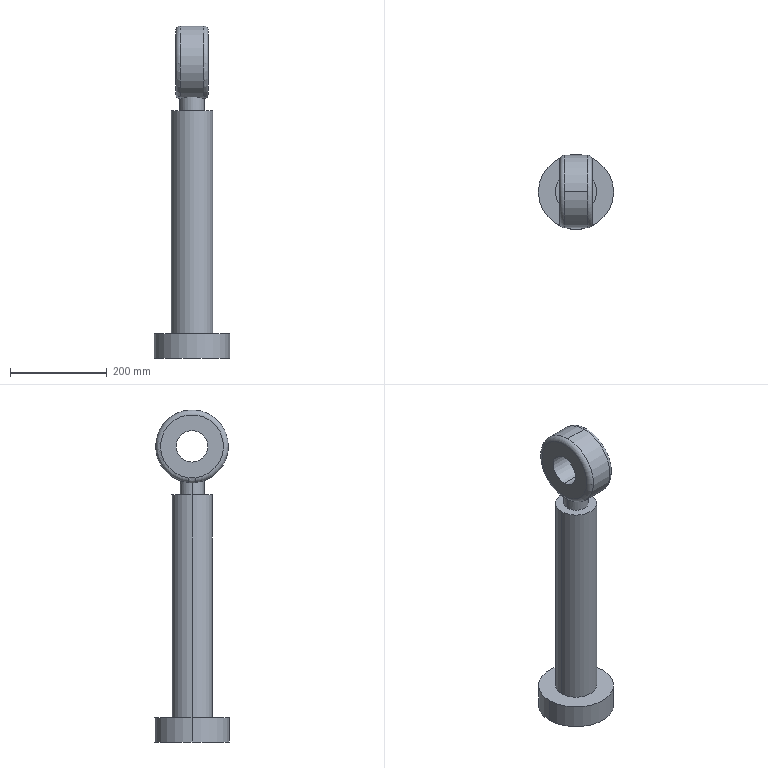Part | SolidWorks | features ICE 3, Extrusion 1, Fillet 1, RevCut 1 | 1 solid | 19 faces | box 155 x 155 x 685 mm | volume 4561292 mm3 | cylinder 10 | plane 5 | torus 2 | spline 2 | commonest cylinder face diameters 50 x2 65 x2 85 x2 150 x2 155 x2
STEP:
#1=CARTESIAN_POINT('',(34.,0.,592.5));
#2=VERTEX_POINT('',#1);
#3=CARTESIAN_POINT('',(34.,0.,527.5));
#4=VERTEX_POINT('',#3);
#5=CARTESIAN_POINT('',(34.,0.,560.));
#6=DIRECTION('',(1.,0.,0.));
#7=DIRECTION('',(0.,0.,-1.));
#8=AXIS2_PLACEMENT_3D('',#5,#6,#7);
#9=CIRCLE('',#8,32.5);
#10=EDGE_CURVE('',#2,#4,#9,.T.);
#11=ORIENTED_EDGE('',*,*,#10,.T.);
#12=CARTESIAN_POINT('',(-34.,0.,527.5));
#13=VERTEX_POINT('',#12);
#14=CARTESIAN_POINT('',(34.,0.,527.5));
#15=DIRECTION('',(-1.,0.,0.));
#16=VECTOR('',#15,1000.);
#17=LINE('',#14,#16);
#18=EDGE_CURVE('',#4,#13,#17,.T.);
#19=ORIENTED_EDGE('',*,*,#18,.T.);
#20=CARTESIAN_POINT('',(-34.,0.,592.5));
#21=VERTEX_POINT('',#20);
#22=CARTESIAN_POINT('',(-34.,0.,560.));
#23=DIRECTION('',(1.,0.,0.));
#24=DIRECTION('',(0.,0.,-1.));
#25=AXIS2_PLACEMENT_3D('',#22,#23,#24);
#26=CIRCLE('',#25,32.5);
#27=EDGE_CURVE('',#21,#13,#26,.T.);
#28=ORIENTED_EDGE('',*,*,#27,.F.);
#29=CARTESIAN_POINT('',(34.,0.,592.5));
#30=DIRECTION('',(-1.,0.,0.));
#31=VECTOR('',#30,1000.);
#32=LINE('',#29,#31);
#33=EDGE_CURVE('',#2,#21,#32,.T.);
#34=ORIENTED_EDGE('',*,*,#33,.F.);
#35=EDGE_LOOP('',(#11,#19,#28,#34));
#36=FACE_OUTER_BOUND('',#35,.T.);
#37=CARTESIAN_POINT('',(34.,0.,560.));
#38=DIRECTION('',(-1.,0.,0.));
#39=DIRECTION('',(0.,0.,1.));
#40=AXIS2_PLACEMENT_3D('',#37,#38,#39);
#41=CYLINDRICAL_SURFACE('',#40,32.5);
#42=ADVANCED_FACE('',(#36),#41,.F.);
#43=CARTESIAN_POINT('',(24.,-7.,485.327));
#44=VERTEX_POINT('',#43);
#45=CARTESIAN_POINT('',(24.,0.,635.));
#46=VERTEX_POINT('',#45);
#47=CARTESIAN_POINT('',(24.,0.,560.));
#48=DIRECTION('',(-1.,0.,0.));
#49=DIRECTION('',(0.,0.,-1.));
#50=AXIS2_PLACEMENT_3D('',#47,#48,#49);
#51=CIRCLE('',#50,75.);
#52=EDGE_CURVE('',#44,#46,#51,.T.);
#53=ORIENTED_EDGE('',*,*,#52,.T.);
#54=CARTESIAN_POINT('',(-24.,0.,635.));
#55=VERTEX_POINT('',#54);
#56=CARTESIAN_POINT('',(34.,0.,635.));
#57=DIRECTION('',(-1.,0.,0.));
#58=VECTOR('',#57,1000.);
#59=LINE('',#56,#58);
#60=EDGE_CURVE('',#46,#55,#59,.T.);
#61=ORIENTED_EDGE('',*,*,#60,.T.);
#62=CARTESIAN_POINT('',(-24.,-7.,485.327));
#63=VERTEX_POINT('',#62);
#64=CARTESIAN_POINT('',(-24.,0.,560.));
#65=DIRECTION('',(1.,0.,0.));
#66=DIRECTION('',(0.,0.,-1.));
#67=AXIS2_PLACEMENT_3D('',#64,#65,#66);
#68=CIRCLE('',#67,75.);
#69=EDGE_CURVE('',#55,#63,#68,.T.);
#70=ORIENTED_EDGE('',*,*,#69,.T.);
#71=CARTESIAN_POINT('',(-24.,-7.,485.327));
#72=CARTESIAN_POINT('',(-23.811,-7.648,485.388));
#73=CARTESIAN_POINT('',(-23.594,-8.294,485.457));
#74=CARTESIAN_POINT('',(-23.112,-9.554,485.608));
#75=CARTESIAN_POINT('',(-22.847,-10.171,485.69));
#76=CARTESIAN_POINT('',(-21.983,-11.98,485.953));
#77=CARTESIAN_POINT('',(-21.315,-13.133,486.15));
#78=CARTESIAN_POINT('',(-20.171,-14.785,486.47));
#79=CARTESIAN_POINT('',(-19.764,-15.324,486.58));
#80=CARTESIAN_POINT('',(-18.916,-16.36,486.804));
#81=CARTESIAN_POINT('',(-18.473,-16.858,486.917));
#82=CARTESIAN_POINT('',(-17.091,-18.294,487.259));
#83=CARTESIAN_POINT('',(-16.098,-19.174,487.488));
#84=CARTESIAN_POINT('',(-14.497,-20.379,487.821));
#85=CARTESIAN_POINT('',(-13.942,-20.763,487.93));
#86=CARTESIAN_POINT('',(-12.807,-21.481,488.141));
#87=CARTESIAN_POINT('',(-12.228,-21.816,488.242));
#88=CARTESIAN_POINT('',(-10.457,-22.747,488.53));
#89=CARTESIAN_POINT('',(-9.231,-23.272,488.7));
#90=CARTESIAN_POINT('',(-7.322,-23.913,488.914));
#91=CARTESIAN_POINT('',(-6.674,-24.102,488.978));
#92=CARTESIAN_POINT('',(-5.353,-24.43,489.09));
#93=CARTESIAN_POINT('',(-4.69,-24.565,489.137));
#94=CARTESIAN_POINT('',(-2.695,-24.891,489.25));
#95=CARTESIAN_POINT('',(-1.356,-25.,489.289));
#96=CARTESIAN_POINT('',(0.6674,-25.,489.289));
#97=CARTESIAN_POINT('',(1.344,-24.973,489.28));
#98=CARTESIAN_POINT('',(2.702,-24.863,489.241));
#99=CARTESIAN_POINT('',(3.378,-24.78,489.212));
#100=CARTESIAN_POINT('',(5.377,-24.452,489.098));
#101=CARTESIAN_POINT('',(6.679,-24.129,488.986));
#102=CARTESIAN_POINT('',(8.59,-23.488,488.772));
#103=CARTESIAN_POINT('',(9.219,-23.248,488.694));
#104=CARTESIAN_POINT('',(10.463,-22.715,488.522));
#105=CARTESIAN_POINT('',(11.071,-22.425,488.43));
#106=CARTESIAN_POINT('',(12.847,-21.488,488.141));
#107=CARTESIAN_POINT('',(13.97,-20.775,487.93));
#108=CARTESIAN_POINT('',(15.568,-19.573,487.598));
#109=CARTESIAN_POINT('',(16.086,-19.149,487.484));
#110=CARTESIAN_POINT('',(17.091,-18.258,487.255));
#111=CARTESIAN_POINT('',(17.574,-17.793,487.14));
#112=CARTESIAN_POINT('',(18.958,-16.351,486.798));
#113=CARTESIAN_POINT('',(19.798,-15.324,486.574));
#114=CARTESIAN_POINT('',(20.935,-13.681,486.256));
#115=CARTESIAN_POINT('',(21.293,-13.116,486.153));
#116=CARTESIAN_POINT('',(21.968,-11.952,485.956));
#117=CARTESIAN_POINT('',(22.284,-11.353,485.862));
#118=CARTESIAN_POINT('',(23.149,-9.536,485.599));
#119=CARTESIAN_POINT('',(23.625,-8.287,485.448));
#120=CARTESIAN_POINT('',(24.,-7.,485.327));
#121=B_SPLINE_CURVE_WITH_KNOTS('',3,(#71,#72,#73,#74,#75,#76,#77,#78,#79,#80,#81,#82,#83,#84,#85,#86,#87,#88,#89,#90,#91,#92,#93,#94,#95,#96,#97,#98,#99,#100,#101,#102,#103,#104,#105,#106,#107,#108,#109,#110,#111,#112,#113,#114,#115,#116,#117,#118,#119,#120),.UNSPECIFIED.,.F.,.F.,(4,2,2,2,2,2,2,2,2,2,2,2,2,2,2,2,2,2,2,2,2,2,2,2,4),(0.007077,0.009095,0.01111,0.01515,0.01717,0.01919,0.02322,0.02524,0.02726,0.0313,0.03331,0.03533,0.03937,0.04139,0.04341,0.04744,0.04946,0.05148,0.05552,0.05753,0.05955,0.06359,0.06561,0.06763,0.07166),.UNSPECIFIED.);
#122=EDGE_CURVE('',#63,#44,#121,.T.);
#123=ORIENTED_EDGE('',*,*,#122,.T.);
#124=EDGE_LOOP('',(#53,#61,#70,#123));
#125=FACE_OUTER_BOUND('',#124,.T.);
#126=CARTESIAN_POINT('',(34.,0.,560.));
#127=DIRECTION('',(-1.,0.,0.));
#128=DIRECTION('',(0.,0.,1.));
#129=AXIS2_PLACEMENT_3D('',#126,#127,#128);
#130=CYLINDRICAL_SURFACE('',#129,75.);
#131=ADVANCED_FACE('',(#125),#130,.T.);
#132=CARTESIAN_POINT('',(25.,0.,485.));
#133=VERTEX_POINT('',#132);
#134=CARTESIAN_POINT('',(24.,7.,485.327));
#135=VERTEX_POINT('',#134);
#136=CARTESIAN_POINT('',(25.,0.,485.));
#137=CARTESIAN_POINT('',(25.,1.177,485.));
#138=CARTESIAN_POINT('',(24.917,2.354,485.028));
#139=CARTESIAN_POINT('',(24.666,4.118,485.111));
#140=CARTESIAN_POINT('',(24.56,4.707,485.146));
#141=CARTESIAN_POINT('',(24.31,5.864,485.227));
#142=CARTESIAN_POINT('',(24.165,6.436,485.274));
#143=CARTESIAN_POINT('',(24.,7.,485.327));
#144=B_SPLINE_CURVE_WITH_KNOTS('',3,(#136,#137,#138,#139,#140,#141,#142,#143),.UNSPECIFIED.,.F.,.F.,(4,2,2,4),(0.07873,0.08226,0.08403,0.08579),.UNSPECIFIED.);
#145=EDGE_CURVE('',#133,#135,#144,.T.);
#146=ORIENTED_EDGE('',*,*,#145,.F.);
#147=CARTESIAN_POINT('',(25.,0.,460.));
#148=VERTEX_POINT('',#147);
#149=CARTESIAN_POINT('',(25.,0.,635.001));
#150=DIRECTION('',(0.,0.,-1.));
#151=VECTOR('',#150,1000.);
#152=LINE('',#149,#151);
#153=EDGE_CURVE('',#133,#148,#152,.T.);
#154=ORIENTED_EDGE('',*,*,#153,.T.);
#155=CARTESIAN_POINT('',(-25.,0.,460.));
#156=VERTEX_POINT('',#155);
#157=CARTESIAN_POINT('',(0.,0.,460.));
#158=DIRECTION('',(0.,0.,1.));
#159=DIRECTION('',(1.,0.,0.));
#160=AXIS2_PLACEMENT_3D('',#157,#158,#159);
#161=CIRCLE('',#160,25.);
#162=EDGE_CURVE('',#148,#156,#161,.T.);
#163=ORIENTED_EDGE('',*,*,#162,.T.);
#164=CARTESIAN_POINT('',(-25.,0.,485.));
#165=VERTEX_POINT('',#164);
#166=CARTESIAN_POINT('',(-25.,0.,635.001));
#167=DIRECTION('',(0.,0.,-1.));
#168=VECTOR('',#167,1000.);
#169=LINE('',#166,#168);
#170=EDGE_CURVE('',#165,#156,#169,.T.);
#171=ORIENTED_EDGE('',*,*,#170,.F.);
#172=CARTESIAN_POINT('',(-24.,7.,485.327));
#173=VERTEX_POINT('',#172);
#174=CARTESIAN_POINT('',(-24.,7.,485.327));
#175=CARTESIAN_POINT('',(-24.331,5.864,485.221));
#176=CARTESIAN_POINT('',(-24.58,4.712,485.139));
#177=CARTESIAN_POINT('',(-24.914,2.379,485.029));
#178=CARTESIAN_POINT('',(-25.,1.197,485.));
#179=CARTESIAN_POINT('',(-25.,0.,485.));
#180=B_SPLINE_CURVE_WITH_KNOTS('',3,(#174,#175,#176,#177,#178,#179),.UNSPECIFIED.,.F.,.F.,(4,2,4),(0.1504,0.1539,0.1574),.UNSPECIFIED.);
#181=EDGE_CURVE('',#173,#165,#180,.T.);
#182=ORIENTED_EDGE('',*,*,#181,.F.);
#183=CARTESIAN_POINT('',(24.,7.,485.327));
#184=CARTESIAN_POINT('',(23.624,8.289,485.448));
#185=CARTESIAN_POINT('',(23.147,9.54,485.599));
#186=CARTESIAN_POINT('',(22.279,11.361,485.863));
#187=CARTESIAN_POINT('',(21.963,11.961,485.958));
#188=CARTESIAN_POINT('',(21.289,13.123,486.155));
#189=CARTESIAN_POINT('',(20.931,13.687,486.257));
#190=CARTESIAN_POINT('',(19.794,15.329,486.575));
#191=CARTESIAN_POINT('',(18.953,16.358,486.799));
#192=CARTESIAN_POINT('',(17.564,17.803,487.142));
#193=CARTESIAN_POINT('',(17.078,18.27,487.258));
#194=CARTESIAN_POINT('',(16.076,19.158,487.487));
#195=CARTESIAN_POINT('',(15.56,19.579,487.599));
#196=CARTESIAN_POINT('',(13.966,20.778,487.931));
#197=CARTESIAN_POINT('',(12.844,21.49,488.142));
#198=CARTESIAN_POINT('',(11.069,22.426,488.431));
#199=CARTESIAN_POINT('',(10.459,22.717,488.523));
#200=CARTESIAN_POINT('',(9.217,23.249,488.694));
#201=CARTESIAN_POINT('',(8.589,23.488,488.772));
#202=CARTESIAN_POINT('',(6.682,24.128,488.986));
#203=CARTESIAN_POINT('',(5.382,24.451,489.097));
#204=CARTESIAN_POINT('',(3.389,24.778,489.211));
#205=CARTESIAN_POINT('',(2.718,24.861,489.24));
#206=CARTESIAN_POINT('',(1.359,24.972,489.28));
#207=CARTESIAN_POINT('',(0.6788,25.,489.289));
#208=CARTESIAN_POINT('',(-1.348,25.,489.289));
#209=CARTESIAN_POINT('',(-2.689,24.891,489.251));
#210=CARTESIAN_POINT('',(-4.684,24.567,489.137));
#211=CARTESIAN_POINT('',(-5.346,24.431,489.091));
#212=CARTESIAN_POINT('',(-6.665,24.105,488.979));
#213=CARTESIAN_POINT('',(-7.316,23.915,488.915));
#214=CARTESIAN_POINT('',(-9.229,23.273,488.701));
#215=CARTESIAN_POINT('',(-10.457,22.747,488.53));
#216=CARTESIAN_POINT('',(-12.233,21.813,488.241));
#217=CARTESIAN_POINT('',(-12.813,21.477,488.14));
#218=CARTESIAN_POINT('',(-13.952,20.756,487.928));
#219=CARTESIAN_POINT('',(-14.503,20.374,487.819));
#220=CARTESIAN_POINT('',(-16.101,19.171,487.487));
#221=CARTESIAN_POINT('',(-17.094,18.291,487.258));
#222=CARTESIAN_POINT('',(-18.478,16.852,486.916));
#223=CARTESIAN_POINT('',(-18.922,16.353,486.803));
#224=CARTESIAN_POINT('',(-19.773,15.313,486.578));
#225=CARTESIAN_POINT('',(-20.177,14.776,486.468));
#226=CARTESIAN_POINT('',(-21.317,13.129,486.15));
#227=CARTESIAN_POINT('',(-21.984,11.978,485.953));
#228=CARTESIAN_POINT('',(-22.847,10.171,485.69));
#229=CARTESIAN_POINT('',(-23.112,9.554,485.608));
#230=CARTESIAN_POINT('',(-23.594,8.294,485.457));
#231=CARTESIAN_POINT('',(-23.811,7.648,485.388));
#232=CARTESIAN_POINT('',(-24.,7.,485.327));
#233=B_SPLINE_CURVE_WITH_KNOTS('',3,(#183,#184,#185,#186,#187,#188,#189,#190,#191,#192,#193,#194,#195,#196,#197,#198,#199,#200,#201,#202,#203,#204,#205,#206,#207,#208,#209,#210,#211,#212,#213,#214,#215,#216,#217,#218,#219,#220,#221,#222,#223,#224,#225,#226,#227,#228,#229,#230,#231,#232),.UNSPECIFIED.,.F.,.F.,(4,2,2,2,2,2,2,2,2,2,2,2,2,2,2,2,2,2,2,2,2,2,2,2,4),(0.08579,0.08983,0.09185,0.09386,0.0979,0.09992,0.1019,0.106,0.108,0.11,0.114,0.1161,0.1181,0.1221,0.1241,0.1261,0.1302,0.1322,0.1342,0.1383,0.1403,0.1423,0.1463,0.1483,0.1504),.UNSPECIFIED.);
#234=EDGE_CURVE('',#135,#173,#233,.T.);
#235=ORIENTED_EDGE('',*,*,#234,.F.);
#236=EDGE_LOOP('',(#146,#154,#163,#171,#182,#235));
#237=FACE_OUTER_BOUND('',#236,.T.);
#238=CARTESIAN_POINT('',(0.,0.,635.001));
#239=DIRECTION('',(0.,0.,-1.));
#240=DIRECTION('',(-1.,0.,0.));
#241=AXIS2_PLACEMENT_3D('',#238,#239,#240);
#242=CYLINDRICAL_SURFACE('',#241,25.);
#243=ADVANCED_FACE('',(#237),#242,.T.);
#244=CARTESIAN_POINT('',(-77.5,0.,-50.));
#245=VERTEX_POINT('',#244);
#246=CARTESIAN_POINT('',(77.5,0.,-50.));
#247=VERTEX_POINT('',#246);
#248=CARTESIAN_POINT('',(0.,0.,-50.));
#249=DIRECTION('',(0.,0.,-1.));
#250=DIRECTION('',(-1.,0.,0.));
#251=AXIS2_PLACEMENT_3D('',#248,#249,#250);
#252=CIRCLE('',#251,77.5);
#253=EDGE_CURVE('',#245,#247,#252,.T.);
#254=ORIENTED_EDGE('',*,*,#253,.F.);
#255=CARTESIAN_POINT('',(-77.5,0.,0.));
#256=VERTEX_POINT('',#255);
#257=CARTESIAN_POINT('',(-77.5,0.,-50.));
#258=DIRECTION('',(0.,0.,1.));
#259=VECTOR('',#258,1000.);
#260=LINE('',#257,#259);
#261=EDGE_CURVE('',#245,#256,#260,.T.);
#262=ORIENTED_EDGE('',*,*,#261,.T.);
#263=CARTESIAN_POINT('',(77.5,0.,0.));
#264=VERTEX_POINT('',#263);
#265=CARTESIAN_POINT('',(0.,0.,0.));
#266=DIRECTION('',(0.,0.,-1.));
#267=DIRECTION('',(-1.,0.,0.));
#268=AXIS2_PLACEMENT_3D('',#265,#266,#267);
#269=CIRCLE('',#268,77.5);
#270=EDGE_CURVE('',#256,#264,#269,.T.);
#271=ORIENTED_EDGE('',*,*,#270,.T.);
#272=CARTESIAN_POINT('',(77.5,0.,-50.));
#273=DIRECTION('',(0.,0.,1.));
#274=VECTOR('',#273,1000.);
#275=LINE('',#272,#274);
#276=EDGE_CURVE('',#247,#264,#275,.T.);
#277=ORIENTED_EDGE('',*,*,#276,.F.);
#278=EDGE_LOOP('',(#254,#262,#271,#277));
#279=FACE_OUTER_BOUND('',#278,.T.);
#280=CARTESIAN_POINT('',(0.,0.,-50.));
#281=DIRECTION('',(0.,0.,1.));
#282=DIRECTION('',(1.,0.,0.));
#283=AXIS2_PLACEMENT_3D('',#280,#281,#282);
#284=CYLINDRICAL_SURFACE('',#283,77.5);
#285=ADVANCED_FACE('',(#279),#284,.T.);
#286=CARTESIAN_POINT('',(42.5,0.,460.));
#287=VERTEX_POINT('',#286);
#288=CARTESIAN_POINT('',(-42.5,0.,460.));
#289=VERTEX_POINT('',#288);
#290=CARTESIAN_POINT('',(0.,0.,460.));
#291=DIRECTION('',(0.,0.,1.));
#292=DIRECTION('',(1.,0.,0.));
#293=AXIS2_PLACEMENT_3D('',#290,#291,#292);
#294=CIRCLE('',#293,42.5);
#295=EDGE_CURVE('',#287,#289,#294,.T.);
#296=ORIENTED_EDGE('',*,*,#295,.F.);
#297=CARTESIAN_POINT('',(42.5,0.,0.));
#298=VERTEX_POINT('',#297);
#299=CARTESIAN_POINT('',(42.5,0.,460.));
#300=DIRECTION('',(0.,0.,-1.));
#301=VECTOR('',#300,1000.);
#302=LINE('',#299,#301);
#303=EDGE_CURVE('',#287,#298,#302,.T.);
#304=ORIENTED_EDGE('',*,*,#303,.T.);
#305=CARTESIAN_POINT('',(-42.5,0.,0.));
#306=VERTEX_POINT('',#305);
#307=CARTESIAN_POINT('',(0.,0.,0.));
#308=DIRECTION('',(0.,0.,-1.));
#309=DIRECTION('',(-1.,0.,0.));
#310=AXIS2_PLACEMENT_3D('',#307,#308,#309);
#311=CIRCLE('',#310,42.5);
#312=EDGE_CURVE('',#306,#298,#311,.T.);
#313=ORIENTED_EDGE('',*,*,#312,.F.);
#314=CARTESIAN_POINT('',(-42.5,0.,460.));
#315=DIRECTION('',(0.,0.,-1.));
#316=VECTOR('',#315,1000.);
#317=LINE('',#314,#316);
#318=EDGE_CURVE('',#289,#306,#317,.T.);
#319=ORIENTED_EDGE('',*,*,#318,.F.);
#320=EDGE_LOOP('',(#296,#304,#313,#319));
#321=FACE_OUTER_BOUND('',#320,.T.);
#322=CARTESIAN_POINT('',(0.,0.,460.));
#323=DIRECTION('',(0.,0.,-1.));
#324=DIRECTION('',(-1.,0.,0.));
#325=AXIS2_PLACEMENT_3D('',#322,#323,#324);
#326=CYLINDRICAL_SURFACE('',#325,42.5);
#327=ADVANCED_FACE('',(#321),#326,.T.);
#328=ORIENTED_EDGE('',*,*,#303,.F.);
#329=CARTESIAN_POINT('',(0.,0.,460.));
#330=DIRECTION('',(0.,0.,1.));
#331=DIRECTION('',(1.,0.,0.));
#332=AXIS2_PLACEMENT_3D('',#329,#330,#331);
#333=CIRCLE('',#332,42.5);
#334=EDGE_CURVE('',#289,#287,#333,.T.);
#335=ORIENTED_EDGE('',*,*,#334,.F.);
#336=ORIENTED_EDGE('',*,*,#318,.T.);
#337=CARTESIAN_POINT('',(0.,0.,0.));
#338=DIRECTION('',(0.,0.,-1.));
#339=DIRECTION('',(-1.,0.,0.));
#340=AXIS2_PLACEMENT_3D('',#337,#338,#339);
#341=CIRCLE('',#340,42.5);
#342=EDGE_CURVE('',#298,#306,#341,.T.);
#343=ORIENTED_EDGE('',*,*,#342,.F.);
#344=EDGE_LOOP('',(#328,#335,#336,#343));
#345=FACE_OUTER_BOUND('',#344,.T.);
#346=CARTESIAN_POINT('',(0.,0.,460.));
#347=DIRECTION('',(0.,0.,-1.));
#348=DIRECTION('',(-1.,0.,0.));
#349=AXIS2_PLACEMENT_3D('',#346,#347,#348);
#350=CYLINDRICAL_SURFACE('',#349,42.5);
#351=ADVANCED_FACE('',(#345),#350,.T.);
#352=CARTESIAN_POINT('',(0.,0.,460.));
#353=DIRECTION('',(0.,0.,1.));
#354=DIRECTION('',(1.,0.,0.));
#355=AXIS2_PLACEMENT_3D('',#352,#353,#354);
#356=CIRCLE('',#355,25.);
#357=EDGE_CURVE('',#156,#148,#356,.T.);
#358=ORIENTED_EDGE('',*,*,#357,.F.);
#359=ORIENTED_EDGE('',*,*,#162,.F.);
#360=EDGE_LOOP('',(#358,#359));
#361=FACE_BOUND('',#360,.T.);
#362=ORIENTED_EDGE('',*,*,#334,.T.);
#363=ORIENTED_EDGE('',*,*,#295,.T.);
#364=EDGE_LOOP('',(#362,#363));
#365=FACE_OUTER_BOUND('',#364,.T.);
#366=CARTESIAN_POINT('',(0.,0.,460.));
#367=DIRECTION('',(0.,0.,1.));
#368=DIRECTION('',(1.,0.,0.));
#369=AXIS2_PLACEMENT_3D('',#366,#367,#368);
#370=PLANE('',#369);
#371=ADVANCED_FACE('',(#361,#365),#370,.T.);
#372=ORIENTED_EDGE('',*,*,#261,.F.);
#373=CARTESIAN_POINT('',(0.,0.,-50.));
#374=DIRECTION('',(0.,0.,-1.));
#375=DIRECTION('',(-1.,0.,0.));
#376=AXIS2_PLACEMENT_3D('',#373,#374,#375);
#377=CIRCLE('',#376,77.5);
#378=EDGE_CURVE('',#247,#245,#377,.T.);
#379=ORIENTED_EDGE('',*,*,#378,.F.);
#380=ORIENTED_EDGE('',*,*,#276,.T.);
#381=CARTESIAN_POINT('',(0.,0.,0.));
#382=DIRECTION('',(0.,0.,-1.));
#383=DIRECTION('',(-1.,0.,0.));
#384=AXIS2_PLACEMENT_3D('',#381,#382,#383);
#385=CIRCLE('',#384,77.5);
#386=EDGE_CURVE('',#264,#256,#385,.T.);
#387=ORIENTED_EDGE('',*,*,#386,.T.);
#388=EDGE_LOOP('',(#372,#379,#380,#387));
#389=FACE_OUTER_BOUND('',#388,.T.);
#390=CARTESIAN_POINT('',(0.,0.,-50.));
#391=DIRECTION('',(0.,0.,1.));
#392=DIRECTION('',(1.,0.,0.));
#393=AXIS2_PLACEMENT_3D('',#390,#391,#392);
#394=CYLINDRICAL_SURFACE('',#393,77.5);
#395=ADVANCED_FACE('',(#389),#394,.T.);
#396=ORIENTED_EDGE('',*,*,#378,.T.);
#397=ORIENTED_EDGE('',*,*,#253,.T.);
#398=EDGE_LOOP('',(#396,#397));
#399=FACE_OUTER_BOUND('',#398,.T.);
#400=CARTESIAN_POINT('',(0.,0.,-50.));
#401=DIRECTION('',(0.,0.,-1.));
#402=DIRECTION('',(-1.,0.,0.));
#403=AXIS2_PLACEMENT_3D('',#400,#401,#402);
#404=PLANE('',#403);
#405=ADVANCED_FACE('',(#399),#404,.T.);
#406=ORIENTED_EDGE('',*,*,#312,.T.);
#407=ORIENTED_EDGE('',*,*,#342,.T.);
#408=EDGE_LOOP('',(#406,#407));
#409=FACE_BOUND('',#408,.T.);
#410=ORIENTED_EDGE('',*,*,#386,.F.);
#411=ORIENTED_EDGE('',*,*,#270,.F.);
#412=EDGE_LOOP('',(#410,#411));
#413=FACE_OUTER_BOUND('',#412,.T.);
#414=CARTESIAN_POINT('',(0.,0.,0.));
#415=DIRECTION('',(0.,0.,-1.));
#416=DIRECTION('',(-1.,0.,0.));
#417=AXIS2_PLACEMENT_3D('',#414,#415,#416);
#418=PLANE('',#417);
#419=ADVANCED_FACE('',(#409,#413),#418,.F.);
#420=ORIENTED_EDGE('',*,*,#153,.F.);
#421=CARTESIAN_POINT('',(24.,-7.,485.327));
#422=CARTESIAN_POINT('',(24.164,-6.437,485.275));
#423=CARTESIAN_POINT('',(24.309,-5.867,485.228));
#424=CARTESIAN_POINT('',(24.559,-4.711,485.146));
#425=CARTESIAN_POINT('',(24.665,-4.123,485.111));
#426=CARTESIAN_POINT('',(24.917,-2.355,485.028));
#427=CARTESIAN_POINT('',(25.,-1.177,485.));
#428=CARTESIAN_POINT('',(25.,0.,485.));
#429=B_SPLINE_CURVE_WITH_KNOTS('',3,(#421,#422,#423,#424,#425,#426,#427,#428),.UNSPECIFIED.,.F.,.F.,(4,2,2,4),(0.07166,0.07343,0.0752,0.07873),.UNSPECIFIED.);
#430=EDGE_CURVE('',#44,#133,#429,.T.);
#431=ORIENTED_EDGE('',*,*,#430,.F.);
#432=ORIENTED_EDGE('',*,*,#122,.F.);
#433=CARTESIAN_POINT('',(-25.,0.,485.));
#434=CARTESIAN_POINT('',(-25.,-1.197,485.));
#435=CARTESIAN_POINT('',(-24.914,-2.379,485.029));
#436=CARTESIAN_POINT('',(-24.58,-4.712,485.139));
#437=CARTESIAN_POINT('',(-24.332,-5.863,485.221));
#438=CARTESIAN_POINT('',(-24.,-7.,485.327));
#439=B_SPLINE_CURVE_WITH_KNOTS('',3,(#433,#434,#435,#436,#437,#438),.UNSPECIFIED.,.F.,.F.,(4,2,4),(0.,0.003538,0.007077),.UNSPECIFIED.);
#440=EDGE_CURVE('',#165,#63,#439,.T.);
#441=ORIENTED_EDGE('',*,*,#440,.F.);
#442=ORIENTED_EDGE('',*,*,#170,.T.);
#443=ORIENTED_EDGE('',*,*,#357,.T.);
#444=EDGE_LOOP('',(#420,#431,#432,#441,#442,#443));
#445=FACE_OUTER_BOUND('',#444,.T.);
#446=CARTESIAN_POINT('',(0.,0.,635.001));
#447=DIRECTION('',(0.,0.,-1.));
#448=DIRECTION('',(-1.,0.,0.));
#449=AXIS2_PLACEMENT_3D('',#446,#447,#448);
#450=CYLINDRICAL_SURFACE('',#449,25.);
#451=ADVANCED_FACE('',(#445),#450,.T.);
#452=ORIENTED_EDGE('',*,*,#60,.F.);
#453=CARTESIAN_POINT('',(24.,0.,560.));
#454=DIRECTION('',(-1.,0.,0.));
#455=DIRECTION('',(0.,0.,-1.));
#456=AXIS2_PLACEMENT_3D('',#453,#454,#455);
#457=CIRCLE('',#456,75.);
#458=EDGE_CURVE('',#46,#135,#457,.T.);
#459=ORIENTED_EDGE('',*,*,#458,.T.);
#460=ORIENTED_EDGE('',*,*,#234,.T.);
#461=CARTESIAN_POINT('',(-24.,0.,560.));
#462=DIRECTION('',(1.,0.,0.));
#463=DIRECTION('',(0.,0.,-1.));
#464=AXIS2_PLACEMENT_3D('',#461,#462,#463);
#465=CIRCLE('',#464,75.);
#466=EDGE_CURVE('',#173,#55,#465,.T.);
#467=ORIENTED_EDGE('',*,*,#466,.T.);
#468=EDGE_LOOP('',(#452,#459,#460,#467));
#469=FACE_OUTER_BOUND('',#468,.T.);
#470=CARTESIAN_POINT('',(34.,0.,560.));
#471=DIRECTION('',(-1.,0.,0.));
#472=DIRECTION('',(0.,0.,1.));
#473=AXIS2_PLACEMENT_3D('',#470,#471,#472);
#474=CYLINDRICAL_SURFACE('',#473,75.);
#475=ADVANCED_FACE('',(#469),#474,.T.);
#476=CARTESIAN_POINT('',(34.,6.067,495.284));
#477=VERTEX_POINT('',#476);
#478=CARTESIAN_POINT('',(34.,-6.067,495.284));
#479=VERTEX_POINT('',#478);
#480=CARTESIAN_POINT('',(34.,0.,560.));
#481=DIRECTION('',(1.,0.,0.));
#482=DIRECTION('',(0.,0.,-1.));
#483=AXIS2_PLACEMENT_3D('',#480,#481,#482);
#484=CIRCLE('',#483,65.);
#485=EDGE_CURVE('',#477,#479,#484,.T.);
#486=ORIENTED_EDGE('',*,*,#485,.T.);
#487=CARTESIAN_POINT('',(34.,-6.067,495.284));
#488=CARTESIAN_POINT('',(34.,-5.056,495.189));
#489=CARTESIAN_POINT('',(34.,-4.044,495.103));
#490=CARTESIAN_POINT('',(34.,-2.022,494.983));
#491=CARTESIAN_POINT('',(34.,0.,494.917));
#492=CARTESIAN_POINT('',(34.,2.022,494.983));
#493=CARTESIAN_POINT('',(34.,4.044,495.103));
#494=CARTESIAN_POINT('',(34.,5.056,495.189));
#495=CARTESIAN_POINT('',(34.,6.067,495.284));
#496=B_SPLINE_CURVE_WITH_KNOTS('',3,(#487,#488,#489,#490,#491,#492,#493,#494,#495),.UNSPECIFIED.,.F.,.F.,(4,2,1,2,4),(0.,0.003033,0.006067,0.0091,0.01213),.UNSPECIFIED.);
#497=EDGE_CURVE('',#479,#477,#496,.T.);
#498=ORIENTED_EDGE('',*,*,#497,.T.);
#499=EDGE_LOOP('',(#486,#498));
#500=FACE_OUTER_BOUND('',#499,.T.);
#501=ORIENTED_EDGE('',*,*,#10,.F.);
#502=CARTESIAN_POINT('',(34.,0.,560.));
#503=DIRECTION('',(1.,0.,0.));
#504=DIRECTION('',(0.,0.,-1.));
#505=AXIS2_PLACEMENT_3D('',#502,#503,#504);
#506=CIRCLE('',#505,32.5);
#507=EDGE_CURVE('',#4,#2,#506,.T.);
#508=ORIENTED_EDGE('',*,*,#507,.F.);
#509=EDGE_LOOP('',(#501,#508));
#510=FACE_BOUND('',#509,.T.);
#511=CARTESIAN_POINT('',(34.,0.,560.));
#512=DIRECTION('',(1.,0.,0.));
#513=DIRECTION('',(0.,0.,-1.));
#514=AXIS2_PLACEMENT_3D('',#511,#512,#513);
#515=PLANE('',#514);
#516=ADVANCED_FACE('',(#500,#510),#515,.T.);
#517=CARTESIAN_POINT('',(-34.,6.067,495.284));
#518=VERTEX_POINT('',#517);
#519=CARTESIAN_POINT('',(-34.,-6.067,495.284));
#520=VERTEX_POINT('',#519);
#521=CARTESIAN_POINT('',(-34.,6.067,495.284));
#522=CARTESIAN_POINT('',(-34.,5.056,495.189));
#523=CARTESIAN_POINT('',(-34.,4.044,495.103));
#524=CARTESIAN_POINT('',(-34.,2.022,494.983));
#525=CARTESIAN_POINT('',(-34.,0.,494.917));
#526=CARTESIAN_POINT('',(-34.,-2.022,494.983));
#527=CARTESIAN_POINT('',(-34.,-4.044,495.103));
#528=CARTESIAN_POINT('',(-34.,-5.056,495.189));
#529=CARTESIAN_POINT('',(-34.,-6.067,495.284));
#530=B_SPLINE_CURVE_WITH_KNOTS('',3,(#521,#522,#523,#524,#525,#526,#527,#528,#529),.UNSPECIFIED.,.F.,.F.,(4,2,1,2,4),(0.,0.003033,0.006067,0.0091,0.01213),.UNSPECIFIED.);
#531=EDGE_CURVE('',#518,#520,#530,.T.);
#532=ORIENTED_EDGE('',*,*,#531,.T.);
#533=CARTESIAN_POINT('',(-34.,0.,560.));
#534=DIRECTION('',(-1.,0.,0.));
#535=DIRECTION('',(0.,0.,-1.));
#536=AXIS2_PLACEMENT_3D('',#533,#534,#535);
#537=CIRCLE('',#536,65.);
#538=EDGE_CURVE('',#520,#518,#537,.T.);
#539=ORIENTED_EDGE('',*,*,#538,.T.);
#540=EDGE_LOOP('',(#532,#539));
#541=FACE_OUTER_BOUND('',#540,.T.);
#542=ORIENTED_EDGE('',*,*,#27,.T.);
#543=CARTESIAN_POINT('',(-34.,0.,560.));
#544=DIRECTION('',(1.,0.,0.));
#545=DIRECTION('',(0.,0.,-1.));
#546=AXIS2_PLACEMENT_3D('',#543,#544,#545);
#547=CIRCLE('',#546,32.5);
#548=EDGE_CURVE('',#13,#21,#547,.T.);
#549=ORIENTED_EDGE('',*,*,#548,.T.);
#550=EDGE_LOOP('',(#542,#549));
#551=FACE_BOUND('',#550,.T.);
#552=CARTESIAN_POINT('',(-34.,0.,560.));
#553=DIRECTION('',(1.,0.,0.));
#554=DIRECTION('',(0.,0.,-1.));
#555=AXIS2_PLACEMENT_3D('',#552,#553,#554);
#556=PLANE('',#555);
#557=ADVANCED_FACE('',(#541,#551),#556,.F.);
#558=ORIENTED_EDGE('',*,*,#18,.F.);
#559=ORIENTED_EDGE('',*,*,#507,.T.);
#560=ORIENTED_EDGE('',*,*,#33,.T.);
#561=ORIENTED_EDGE('',*,*,#548,.F.);
#562=EDGE_LOOP('',(#558,#559,#560,#561));
#563=FACE_OUTER_BOUND('',#562,.T.);
#564=CARTESIAN_POINT('',(34.,0.,560.));
#565=DIRECTION('',(-1.,0.,0.));
#566=DIRECTION('',(0.,0.,1.));
#567=AXIS2_PLACEMENT_3D('',#564,#565,#566);
#568=CYLINDRICAL_SURFACE('',#567,32.5);
#569=ADVANCED_FACE('',(#563),#568,.F.);
#570=CARTESIAN_POINT('',(-24.,6.067,495.284));
#571=DIRECTION('',(0.,-0.9956,-0.09333));
#572=DIRECTION('',(0.,0.09333,-0.9956));
#573=AXIS2_PLACEMENT_3D('',#570,#571,#572);
#574=CIRCLE('',#573,10.);
#575=EDGE_CURVE('',#518,#173,#574,.T.);
#576=ORIENTED_EDGE('',*,*,#575,.F.);
#577=ORIENTED_EDGE('',*,*,#538,.F.);
#578=CARTESIAN_POINT('',(-24.,-6.067,495.284));
#579=DIRECTION('',(0.,0.9956,-0.09333));
#580=DIRECTION('',(0.,0.09333,0.9956));
#581=AXIS2_PLACEMENT_3D('',#578,#579,#580);
#582=CIRCLE('',#581,10.);
#583=EDGE_CURVE('',#63,#520,#582,.T.);
#584=ORIENTED_EDGE('',*,*,#583,.F.);
#585=ORIENTED_EDGE('',*,*,#69,.F.);
#586=ORIENTED_EDGE('',*,*,#466,.F.);
#587=EDGE_LOOP('',(#576,#577,#584,#585,#586));
#588=FACE_OUTER_BOUND('',#587,.T.);
#589=CARTESIAN_POINT('',(-24.,0.,560.));
#590=DIRECTION('',(1.,0.,0.));
#591=DIRECTION('',(0.,0.,-1.));
#592=AXIS2_PLACEMENT_3D('',#589,#590,#591);
#593=TOROIDAL_SURFACE('',#592,65.,10.);
#594=ADVANCED_FACE('',(#588),#593,.T.);
#595=ORIENTED_EDGE('',*,*,#583,.T.);
#596=ORIENTED_EDGE('',*,*,#531,.F.);
#597=ORIENTED_EDGE('',*,*,#575,.T.);
#598=ORIENTED_EDGE('',*,*,#181,.T.);
#599=ORIENTED_EDGE('',*,*,#440,.T.);
#600=EDGE_LOOP('',(#595,#596,#597,#598,#599));
#601=FACE_OUTER_BOUND('',#600,.T.);
#602=CARTESIAN_POINT('',(-34.,-6.067,495.284));
#603=CARTESIAN_POINT('',(-34.,-7.,485.327));
#604=CARTESIAN_POINT('',(-24.,-7.,485.327));
#605=CARTESIAN_POINT('',(-34.,-5.056,495.189));
#606=CARTESIAN_POINT('',(-34.,-5.925,485.533));
#607=CARTESIAN_POINT('',(-24.31,-5.938,485.228));
#608=CARTESIAN_POINT('',(-34.,-4.045,495.103));
#609=CARTESIAN_POINT('',(-34.,-4.769,485.677));
#610=CARTESIAN_POINT('',(-24.563,-4.803,485.145));
#611=CARTESIAN_POINT('',(-34.,-2.024,494.983));
#612=CARTESIAN_POINT('',(-34.,-2.417,485.861));
#613=CARTESIAN_POINT('',(-24.909,-2.446,485.031));
#614=CARTESIAN_POINT('',(-34.,-1.013,494.95));
#615=CARTESIAN_POINT('',(-34.,-1.205,485.904));
#616=CARTESIAN_POINT('',(-25.,-1.224,485.));
#617=CARTESIAN_POINT('',(-34.,1.009,494.95));
#618=CARTESIAN_POINT('',(-34.,1.201,485.905));
#619=CARTESIAN_POINT('',(-25.,1.22,485.));
#620=CARTESIAN_POINT('',(-34.,2.021,494.983));
#621=CARTESIAN_POINT('',(-34.,2.413,485.861));
#622=CARTESIAN_POINT('',(-24.909,2.442,485.03));
#623=CARTESIAN_POINT('',(-34.,4.043,495.103));
#624=CARTESIAN_POINT('',(-34.,4.767,485.678));
#625=CARTESIAN_POINT('',(-24.564,4.8,485.144));
#626=CARTESIAN_POINT('',(-34.,5.055,495.189));
#627=CARTESIAN_POINT('',(-34.,5.924,485.533));
#628=CARTESIAN_POINT('',(-24.31,5.937,485.228));
#629=CARTESIAN_POINT('',(-34.,6.067,495.284));
#630=CARTESIAN_POINT('',(-34.,7.,485.327));
#631=CARTESIAN_POINT('',(-24.,7.,485.327));
#632=(BOUNDED_SURFACE()B_SPLINE_SURFACE(3,2,((#602,#603,#604),(#605,#606,#607),(#608,#609,#610),(#611,#612,#613),(#614,#615,#616),(#617,#618,#619),(#620,#621,#622),(#623,#624,#625),(#626,#627,#628),(#629,#630,#631)),.UNSPECIFIED.,.F.,.F.,.F.)B_SPLINE_SURFACE_WITH_KNOTS((4,2,2,2,4),(3,3),(0.02197,0.02499,0.028,0.03102,0.03404),(0.,1.),.UNSPECIFIED.)GEOMETRIC_REPRESENTATION_ITEM()RATIONAL_B_SPLINE_SURFACE(((1.,0.7071,1.),(1.,0.7181,1.),(1.,0.7268,1.),(1.,0.7386,1.),(1.,0.7416,1.),(1.,0.7416,1.),(1.,0.7386,1.),(1.,0.7268,1.),(1.,0.7181,1.),(1.,0.7071,1.)))REPRESENTATION_ITEM('')SURFACE());
#633=ADVANCED_FACE('',(#601),#632,.T.);
#634=CARTESIAN_POINT('',(24.,6.067,495.284));
#635=DIRECTION('',(0.,-0.9956,-0.09333));
#636=DIRECTION('',(0.,0.09333,-0.9956));
#637=AXIS2_PLACEMENT_3D('',#634,#635,#636);
#638=CIRCLE('',#637,10.);
#639=EDGE_CURVE('',#135,#477,#638,.T.);
#640=ORIENTED_EDGE('',*,*,#639,.F.);
#641=ORIENTED_EDGE('',*,*,#458,.F.);
#642=ORIENTED_EDGE('',*,*,#52,.F.);
#643=CARTESIAN_POINT('',(24.,-6.067,495.284));
#644=DIRECTION('',(0.,0.9956,-0.09333));
#645=DIRECTION('',(0.,0.09333,0.9956));
#646=AXIS2_PLACEMENT_3D('',#643,#644,#645);
#647=CIRCLE('',#646,10.);
#648=EDGE_CURVE('',#479,#44,#647,.T.);
#649=ORIENTED_EDGE('',*,*,#648,.F.);
#650=ORIENTED_EDGE('',*,*,#485,.F.);
#651=EDGE_LOOP('',(#640,#641,#642,#649,#650));
#652=FACE_OUTER_BOUND('',#651,.T.);
#653=CARTESIAN_POINT('',(24.,0.,560.));
#654=DIRECTION('',(1.,0.,0.));
#655=DIRECTION('',(0.,0.,-1.));
#656=AXIS2_PLACEMENT_3D('',#653,#654,#655);
#657=TOROIDAL_SURFACE('',#656,65.,10.);
#658=ADVANCED_FACE('',(#652),#657,.T.);
#659=ORIENTED_EDGE('',*,*,#648,.T.);
#660=ORIENTED_EDGE('',*,*,#430,.T.);
#661=ORIENTED_EDGE('',*,*,#145,.T.);
#662=ORIENTED_EDGE('',*,*,#639,.T.);
#663=ORIENTED_EDGE('',*,*,#497,.F.);
#664=EDGE_LOOP('',(#659,#660,#661,#662,#663));
#665=FACE_OUTER_BOUND('',#664,.T.);
#666=CARTESIAN_POINT('',(34.,6.067,495.284));
#667=CARTESIAN_POINT('',(34.,7.,485.327));
#668=CARTESIAN_POINT('',(24.,7.,485.327));
#669=CARTESIAN_POINT('',(34.,5.056,495.189));
#670=CARTESIAN_POINT('',(34.,5.925,485.533));
#671=CARTESIAN_POINT('',(24.31,5.938,485.228));
#672=CARTESIAN_POINT('',(34.,4.045,495.103));
#673=CARTESIAN_POINT('',(34.,4.769,485.677));
#674=CARTESIAN_POINT('',(24.563,4.803,485.145));
#675=CARTESIAN_POINT('',(34.,2.024,494.983));
#676=CARTESIAN_POINT('',(34.,2.417,485.861));
#677=CARTESIAN_POINT('',(24.909,2.446,485.031));
#678=CARTESIAN_POINT('',(34.,1.013,494.95));
#679=CARTESIAN_POINT('',(34.,1.205,485.904));
#680=CARTESIAN_POINT('',(25.,1.224,485.));
#681=CARTESIAN_POINT('',(34.,-1.009,494.95));
#682=CARTESIAN_POINT('',(34.,-1.201,485.905));
#683=CARTESIAN_POINT('',(25.,-1.22,485.));
#684=CARTESIAN_POINT('',(34.,-2.021,494.983));
#685=CARTESIAN_POINT('',(34.,-2.413,485.861));
#686=CARTESIAN_POINT('',(24.909,-2.442,485.03));
#687=CARTESIAN_POINT('',(34.,-4.043,495.103));
#688=CARTESIAN_POINT('',(34.,-4.767,485.678));
#689=CARTESIAN_POINT('',(24.564,-4.8,485.144));
#690=CARTESIAN_POINT('',(34.,-5.055,495.189));
#691=CARTESIAN_POINT('',(34.,-5.924,485.533));
#692=CARTESIAN_POINT('',(24.31,-5.937,485.228));
#693=CARTESIAN_POINT('',(34.,-6.067,495.284));
#694=CARTESIAN_POINT('',(34.,-7.,485.327));
#695=CARTESIAN_POINT('',(24.,-7.,485.327));
#696=(BOUNDED_SURFACE()B_SPLINE_SURFACE(3,2,((#666,#667,#668),(#669,#670,#671),(#672,#673,#674),(#675,#676,#677),(#678,#679,#680),(#681,#682,#683),(#684,#685,#686),(#687,#688,#689),(#690,#691,#692),(#693,#694,#695)),.UNSPECIFIED.,.F.,.F.,.F.)B_SPLINE_SURFACE_WITH_KNOTS((4,2,2,2,4),(3,3),(0.02197,0.02499,0.028,0.03102,0.03404),(0.,1.),.UNSPECIFIED.)GEOMETRIC_REPRESENTATION_ITEM()RATIONAL_B_SPLINE_SURFACE(((1.,0.7071,1.),(1.,0.7181,1.),(1.,0.7268,1.),(1.,0.7386,1.),(1.,0.7416,1.),(1.,0.7416,1.),(1.,0.7386,1.),(1.,0.7268,1.),(1.,0.7181,1.),(1.,0.7071,1.)))REPRESENTATION_ITEM('')SURFACE());
#697=ADVANCED_FACE('',(#665),#696,.T.);
#698=CLOSED_SHELL('',(#42,#131,#243,#285,#327,#351,#371,#395,#405,#419,#451,#475,#516,#557,#569,#594,#633,#658,#697));
#699=MANIFOLD_SOLID_BREP('',#698);
#700=CARTESIAN_POINT('',(0.,0.,0.));
#701=DIRECTION('',(0.,0.,1.));
#702=DIRECTION('',(1.,0.,0.));
#703=AXIS2_PLACEMENT_3D('',#700,#701,#702);
#704=(LENGTH_UNIT()NAMED_UNIT(*)SI_UNIT(.MILLI.,.METRE.));
#705=UNCERTAINTY_MEASURE_WITH_UNIT(LENGTH_MEASURE(0.00001),#704,'','');
#706=(NAMED_UNIT(*)PLANE_ANGLE_UNIT()SI_UNIT($,.RADIAN.));
#707=(NAMED_UNIT(*)SI_UNIT($,.STERADIAN.)SOLID_ANGLE_UNIT());
#708=(GEOMETRIC_REPRESENTATION_CONTEXT(3)GLOBAL_UNCERTAINTY_ASSIGNED_CONTEXT((#705))GLOBAL_UNIT_ASSIGNED_CONTEXT((#704,#706,#707))REPRESENTATION_CONTEXT('',''));
#709=ADVANCED_BREP_SHAPE_REPRESENTATION('',(#699,#703),#708);